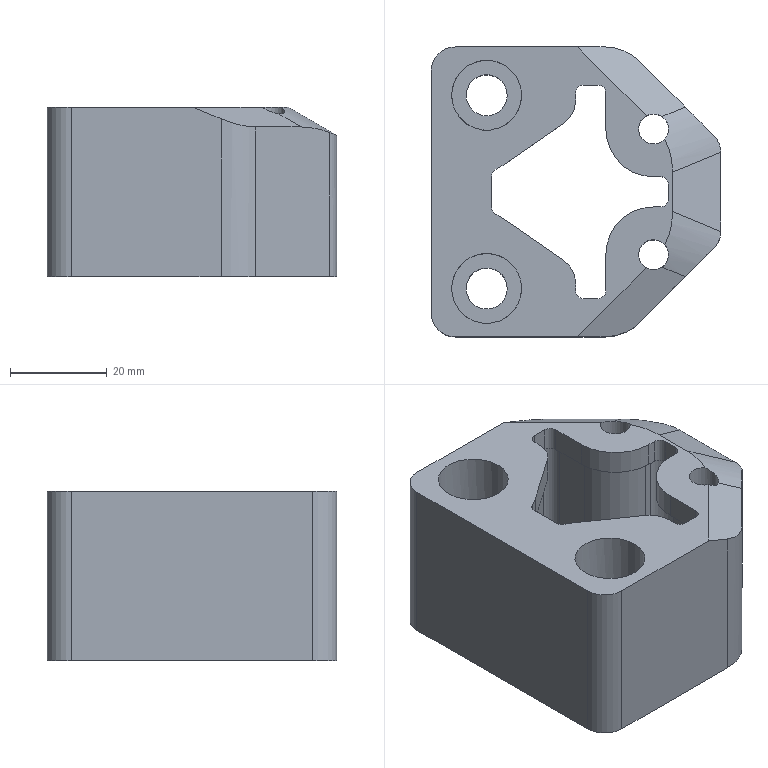Part | NX | features DIE-104 2 | 1 solid | 90 faces | box 60 x 60 x 35 mm | volume 71749 mm3 | cylinder 44 | plane 42 | spline 4 | commonest cylinder face diameters 3.24 x8 5.24 x8 9.76 x4 10 x4 6.201 x2 7.76 x2